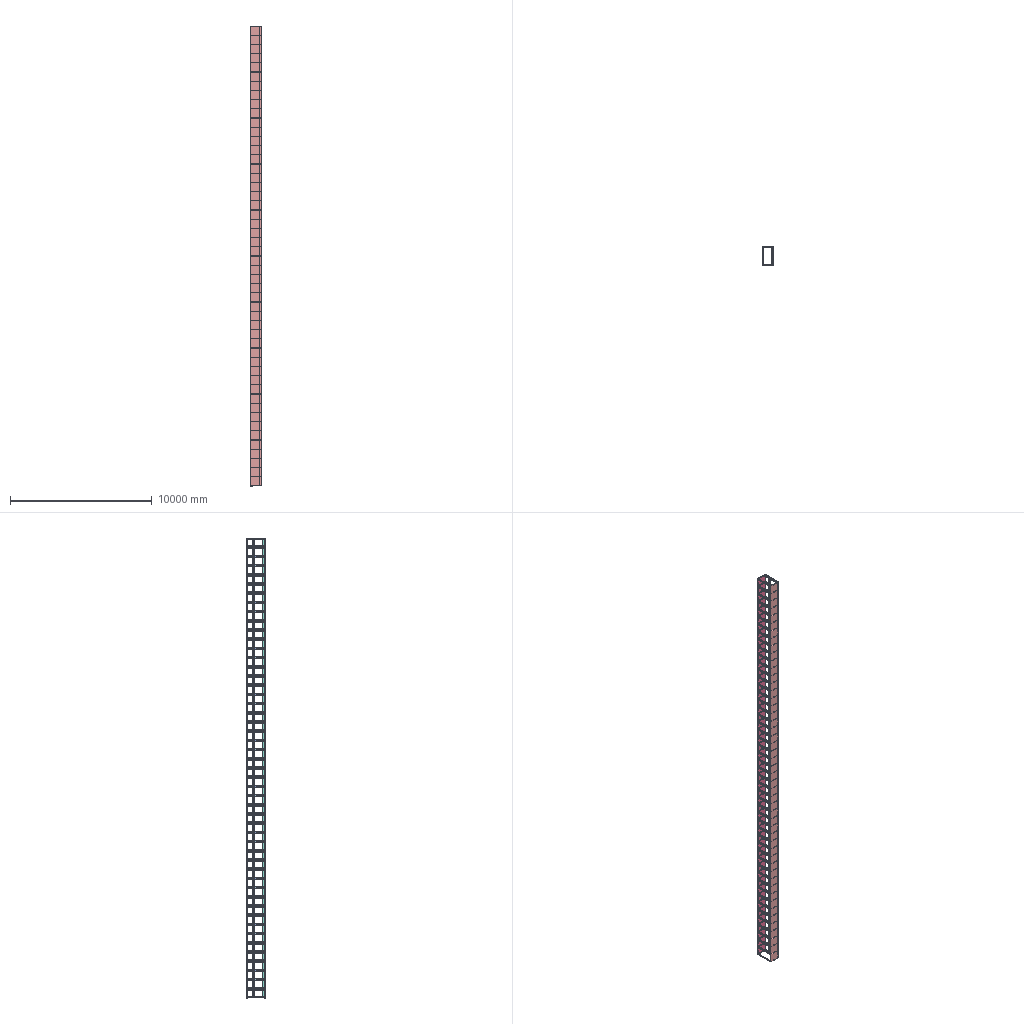Assembly | SolidWorks | 14 different items | 700 placed | box 800 x 1351 x 32500 mm
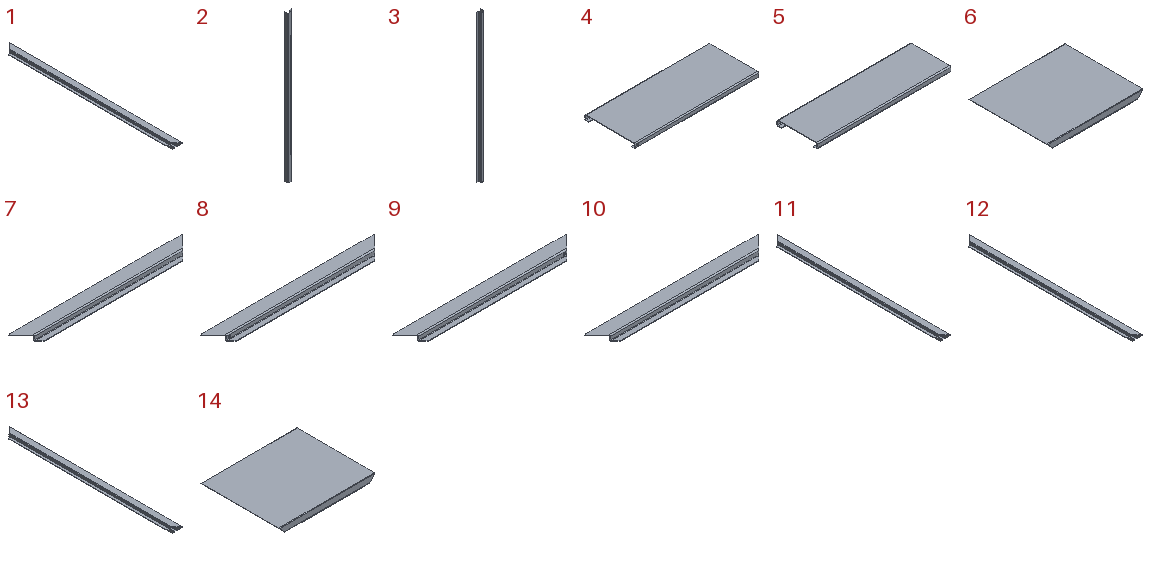Parts list (item | quantity | size | volume | features):
1 | x50 | 68 x 1345 x 68 mm | 416933 mm3 | features EdgeFlange 5, ICE 2, Extrusion 1, FlatPattern 1, SheetMetal 1, SolidToSheetMetal 1
2 | x50 | 51 x 31 x 1331 mm | 252490 mm3 | features ExtruThin 1
3 | x50 | 51 x 31 x 1331 mm | 252490 mm3 | features ExtruThin 1
4 | x50 | 496 x 200 x 20 mm | 254694 mm3 | features EdgeFlange 4, Extrusion 1, FlatPattern 1, ICE 1, SheetMetal 1, SolidToSheetMetal 1
5 | x50 | 496 x 150 x 20 mm | 205094 mm3 | features EdgeFlange 4, Extrusion 1, FlatPattern 1, ICE 1, SheetMetal 1, SolidToSheetMetal 1
6 | x50 | 796 x 650 x 68 mm | 1266578 mm3 | features EdgeFlange 6, Extrusion 1, FlatPattern 1, ICE 1, SheetMetal 1, SolidToSheetMetal 1
7 | x50 | 641.515 x 68 x 20 mm | 96064 mm3 | features EdgeFlange 2, Extrusion 1, Fillet 1, FlatPattern 1, ICE 1, SheetMetal 1, SolidToSheetMetal 1
8 | x50 | 641.515 x 68 x 20 mm | 95964 mm3 | features EdgeFlange 2, ICE 2, Extrusion 1, Fillet 1, FlatPattern 1, SheetMetal 1, SolidToSheetMetal 1
9 | x50 | 641.515 x 68 x 20 mm | 95964 mm3 | features EdgeFlange 2, ICE 2, Extrusion 1, Fillet 1, FlatPattern 1, SheetMetal 1, SolidToSheetMetal 1
10 | x50 | 641.515 x 68 x 20 mm | 96064 mm3 | features EdgeFlange 2, Extrusion 1, Fillet 1, FlatPattern 1, ICE 1, SheetMetal 1, SolidToSheetMetal 1
11 | x50 | 68 x 1345 x 68 mm | 416933 mm3 | features EdgeFlange 5, ICE 2, Extrusion 1, FlatPattern 1, SheetMetal 1, SolidToSheetMetal 1
12 | x50 | 68 x 1345 x 68 mm | 416933 mm3 | features EdgeFlange 5, ICE 2, Extrusion 1, FlatPattern 1, SheetMetal 1, SolidToSheetMetal 1
13 | x50 | 68 x 1349 x 68 mm | 418242 mm3 | features EdgeFlange 5, ICE 2, Extrusion 1, FlatPattern 1, SheetMetal 1, SolidToSheetMetal 1
14 | x50 | 796 x 650 x 68 mm | 1266578 mm3 | features EdgeFlange 6, Extrusion 1, FlatPattern 1, ICE 1, SheetMetal 1, SolidToSheetMetal 1
Mates (type | each side: item.copy, entity, surface, feature):
Coincident | 14.1 face plane UnnamedBody 1 | 2.1 face plane Extrude-Thin Wall1
Coincident | 14.1 face plane UnnamedBody 1 | 3.1 face plane Extrude-Thin Wall1
Coincident | 2.1 face plane Extrude-Thin Wall1 | 3.1 face plane Extrude-Thin Wall1
Coincident | 2.1 face plane Extrude-Thin Wall1 | 4.1 face plane Edge-Flange 2
Coincident | 14.1 face plane UnnamedBody 1 | 4.1 face plane Edge-Flange 1
Coincident | 2.1 face plane Extrude-Thin Wall1 | 4.1 face plane Edge-Flange 3
Coincident | 2.1 face plane Extrude-Thin Wall1 | 5.1 face plane Edge-Flange 2
Coincident | 2.1 face plane Extrude-Thin Wall1 | 5.1 face plane EdgeBend2
DistanceDim | 2.1 face plane Extrude-Thin Wall1 | 9.1 face plane UnnamedBody 1
Coincident | 14.1 face plane Edge-Flange 1 | 11.1 face plane UnnamedBody 1
Coincident | 14.1 face plane Cut-Extrude 1 | 11.1 face plane Cut-Extrude 2
Coincident | 14.1 edge | 11.1 edge
Coincident | 14.1 face plane Edge-Flange 1 | 12.1 face plane Edge-Flange 1 | 2 times
Coincident | 6.1 face plane Edge-Flange 4 | 11.1 face plane UnnamedBody 1
Coincident | 6.1 face plane Cut-Extrude 1 | 11.1 face plane Cut-Extrude 2
Coincident | 6.1 edge | 11.1 edge
Coincident | 8.1 face plane UnnamedBody 1 | 12.1 face plane UnnamedBody 1 | 2 times
Coincident | 14.1 face plane Cut-Extrude 1 | 12.1 face plane Cut-Extrude 1
Coincident | 14.1 edge | 12.1 edge
Coincident | 8.1 face plane Cut-Extrude 1 | 12.1 face plane Cut-Extrude 2
Coincident | 8.1 edge | 12.1 edge
Coincident | 8.1 face plane UnnamedBody 1 | 13.1 face plane UnnamedBody 1
Coincident | 14.1 face plane Edge-Flange 4 | 13.1 face plane Edge-Flange 1
Coincident | 14.1 face plane Cut-Extrude 1 | 13.1 face plane Cut-Extrude 1
Coincident | 9.1 face plane UnnamedBody 1 | 12.1 face plane UnnamedBody 1
Coincident | 14.1 face plane Edge-Flange 4 | 1.1 face plane Edge-Flange 1
Coincident | 1.1 face plane UnnamedBody 1 | 7.1 face plane UnnamedBody 1 | 2 times
Coincident | 14.1 face plane Cut-Extrude 1 | 1.1 face plane Cut-Extrude 1
Coincident | 14.1 edge | 1.1 edge
Coincident | 1.1 face plane Cut-Extrude 2 | 7.1 face plane Cut-Extrude 1
Coincident | 1.1 edge | 7.1 edge
Coincident | 1.1 face plane UnnamedBody 1 | 10.1 face plane UnnamedBody 1
Coincident | 1.1 face plane Cut-Extrude 2 | 10.1 face plane Cut-Extrude 1
Coincident | 1.1 face plane Edge-Flange 5 | 10.1 edge
DistanceDim | 5.1 face plane Edge-Flange 1 | 4.1 face plane Edge-Flange 3
Coincident | 9.1 edge | 12.1 edge
Coincident | 14.1 face plane UnnamedBody 1 | assembly plane